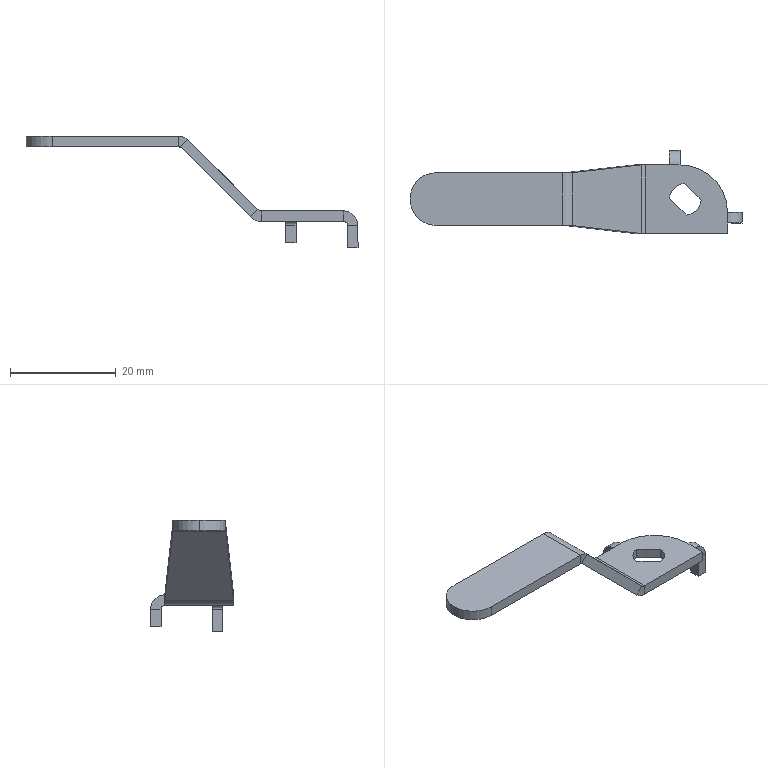Part | SolidWorks | features EdgeFlange 4, Fillet 2, ICE 2, FlatPattern 1, SMBaseFlange 1, SheetMetal 1 | 1 solid | 48 faces | box 62.879 x 15.737 x 21.142 mm | volume 1428 mm3 | plane 35 | cylinder 13 | commonest cylinder face diameters 1.473 x3 5.473 x3 6 x3 10 x2 2 x1 18 x1
STEP:
#1=CARTESIAN_POINT('',(-21.568,5.,13.544));
#2=VERTEX_POINT('',#1);
#3=CARTESIAN_POINT('',(-21.556,5.,13.556));
#4=VERTEX_POINT('',#3);
#5=CARTESIAN_POINT('',(-32.543,5.,2.57));
#6=DIRECTION('',(0.7071,0.,0.7071));
#7=VECTOR('',#6,1000.);
#8=LINE('',#5,#7);
#9=EDGE_CURVE('',#2,#4,#8,.T.);
#10=ORIENTED_EDGE('',*,*,#9,.F.);
#11=CARTESIAN_POINT('',(-21.341,5.,13.341));
#12=VERTEX_POINT('',#11);
#13=CARTESIAN_POINT('',(-23.276,5.,11.406));
#14=DIRECTION('',(0.,1.,0.));
#15=DIRECTION('',(0.,0.,1.));
#16=AXIS2_PLACEMENT_3D('',#13,#14,#15);
#17=CIRCLE('',#16,2.737);
#18=EDGE_CURVE('',#2,#12,#17,.T.);
#19=ORIENTED_EDGE('',*,*,#18,.T.);
#20=CARTESIAN_POINT('',(-4.,5.,-4.));
#21=DIRECTION('',(-0.7071,0.,0.7071));
#22=VECTOR('',#21,1000.);
#23=LINE('',#20,#22);
#24=EDGE_CURVE('',#12,#4,#23,.T.);
#25=ORIENTED_EDGE('',*,*,#24,.T.);
#26=EDGE_LOOP('',(#10,#19,#25));
#27=FACE_OUTER_BOUND('',#26,.T.);
#28=CARTESIAN_POINT('',(-22.971,5.,12.142));
#29=DIRECTION('',(0.,-1.,0.));
#30=DIRECTION('',(0.,0.,-1.));
#31=AXIS2_PLACEMENT_3D('',#28,#29,#30);
#32=PLANE('',#31);
#33=ADVANCED_FACE('',(#27),#32,.T.);
#34=CARTESIAN_POINT('',(-21.556,-5.,13.556));
#35=VERTEX_POINT('',#34);
#36=CARTESIAN_POINT('',(-21.341,-5.,13.341));
#37=VERTEX_POINT('',#36);
#38=CARTESIAN_POINT('',(-4.,-5.,-4.));
#39=DIRECTION('',(0.7071,0.,-0.7071));
#40=VECTOR('',#39,1000.);
#41=LINE('',#38,#40);
#42=EDGE_CURVE('',#35,#37,#41,.T.);
#43=ORIENTED_EDGE('',*,*,#42,.T.);
#44=CARTESIAN_POINT('',(-21.568,-5.,13.544));
#45=VERTEX_POINT('',#44);
#46=CARTESIAN_POINT('',(-23.276,-5.,11.406));
#47=DIRECTION('',(0.,-1.,0.));
#48=DIRECTION('',(0.,0.,1.));
#49=AXIS2_PLACEMENT_3D('',#46,#47,#48);
#50=CIRCLE('',#49,2.737);
#51=EDGE_CURVE('',#37,#45,#50,.T.);
#52=ORIENTED_EDGE('',*,*,#51,.T.);
#53=CARTESIAN_POINT('',(-32.543,-5.,2.57));
#54=DIRECTION('',(0.7071,0.,0.7071));
#55=VECTOR('',#54,1000.);
#56=LINE('',#53,#55);
#57=EDGE_CURVE('',#45,#35,#56,.T.);
#58=ORIENTED_EDGE('',*,*,#57,.T.);
#59=EDGE_LOOP('',(#43,#52,#58));
#60=FACE_OUTER_BOUND('',#59,.T.);
#61=CARTESIAN_POINT('',(-22.755,-5.,11.926));
#62=DIRECTION('',(0.,1.,0.));
#63=DIRECTION('',(0.,0.,1.));
#64=AXIS2_PLACEMENT_3D('',#61,#62,#63);
#65=PLANE('',#64);
#66=ADVANCED_FACE('',(#60),#65,.T.);
#67=CARTESIAN_POINT('',(-22.755,5.,11.926));
#68=VERTEX_POINT('',#67);
#69=CARTESIAN_POINT('',(-22.755,-5.,11.926));
#70=VERTEX_POINT('',#69);
#71=CARTESIAN_POINT('',(-22.755,5.,11.926));
#72=DIRECTION('',(0.,-1.,0.));
#73=VECTOR('',#72,1000.);
#74=LINE('',#71,#73);
#75=EDGE_CURVE('',#68,#70,#74,.T.);
#76=ORIENTED_EDGE('',*,*,#75,.F.);
#77=CARTESIAN_POINT('',(-22.971,5.,12.142));
#78=VERTEX_POINT('',#77);
#79=CARTESIAN_POINT('',(-22.971,5.,12.142));
#80=DIRECTION('',(0.7071,0.,-0.7071));
#81=VECTOR('',#80,1000.);
#82=LINE('',#79,#81);
#83=EDGE_CURVE('',#78,#68,#82,.T.);
#84=ORIENTED_EDGE('',*,*,#83,.F.);
#85=CARTESIAN_POINT('',(-9.707,6.5,-1.121));
#86=VERTEX_POINT('',#85);
#87=CARTESIAN_POINT('',(-9.707,6.5,-1.121));
#88=DIRECTION('',(0.7049,0.07971,-0.7049));
#89=VECTOR('',#88,1000.);
#90=LINE('',#87,#89);
#91=EDGE_CURVE('',#78,#86,#90,.T.);
#92=ORIENTED_EDGE('',*,*,#91,.T.);
#93=CARTESIAN_POINT('',(-9.707,-6.5,-1.121));
#94=VERTEX_POINT('',#93);
#95=CARTESIAN_POINT('',(-9.707,0.,-1.121));
#96=DIRECTION('',(0.,-1.,0.));
#97=VECTOR('',#96,1000.);
#98=LINE('',#95,#97);
#99=EDGE_CURVE('',#86,#94,#98,.T.);
#100=ORIENTED_EDGE('',*,*,#99,.T.);
#101=CARTESIAN_POINT('',(-22.971,-5.,12.142));
#102=VERTEX_POINT('',#101);
#103=CARTESIAN_POINT('',(-9.707,-6.5,-1.121));
#104=DIRECTION('',(-0.7049,0.07971,0.7049));
#105=VECTOR('',#104,1000.);
#106=LINE('',#103,#105);
#107=EDGE_CURVE('',#94,#102,#106,.T.);
#108=ORIENTED_EDGE('',*,*,#107,.T.);
#109=CARTESIAN_POINT('',(-22.755,-5.,11.926));
#110=DIRECTION('',(-0.7071,0.,0.7071));
#111=VECTOR('',#110,1000.);
#112=LINE('',#109,#111);
#113=EDGE_CURVE('',#70,#102,#112,.T.);
#114=ORIENTED_EDGE('',*,*,#113,.F.);
#115=EDGE_LOOP('',(#76,#84,#92,#100,#108,#114));
#116=FACE_OUTER_BOUND('',#115,.T.);
#117=CARTESIAN_POINT('',(-5.414,0.,-5.414));
#118=DIRECTION('',(-0.7071,0.,-0.7071));
#119=DIRECTION('',(-0.7071,0.,0.7071));
#120=AXIS2_PLACEMENT_3D('',#117,#118,#119);
#121=PLANE('',#120);
#122=ADVANCED_FACE('',(#116),#121,.T.);
#123=ORIENTED_EDGE('',*,*,#24,.F.);
#124=CARTESIAN_POINT('',(-21.341,5.,13.341));
#125=DIRECTION('',(0.,-1.,0.));
#126=VECTOR('',#125,1000.);
#127=LINE('',#124,#126);
#128=EDGE_CURVE('',#12,#37,#127,.T.);
#129=ORIENTED_EDGE('',*,*,#128,.T.);
#130=ORIENTED_EDGE('',*,*,#42,.F.);
#131=CARTESIAN_POINT('',(-8.293,-6.5,0.2929));
#132=VERTEX_POINT('',#131);
#133=CARTESIAN_POINT('',(-8.293,-6.5,0.2929));
#134=DIRECTION('',(-0.7049,0.07971,0.7049));
#135=VECTOR('',#134,1000.);
#136=LINE('',#133,#135);
#137=EDGE_CURVE('',#132,#35,#136,.T.);
#138=ORIENTED_EDGE('',*,*,#137,.F.);
#139=CARTESIAN_POINT('',(-8.293,6.5,0.2929));
#140=VERTEX_POINT('',#139);
#141=CARTESIAN_POINT('',(-8.293,6.5,0.2929));
#142=DIRECTION('',(0.,-1.,0.));
#143=VECTOR('',#142,1000.);
#144=LINE('',#141,#143);
#145=EDGE_CURVE('',#140,#132,#144,.T.);
#146=ORIENTED_EDGE('',*,*,#145,.F.);
#147=CARTESIAN_POINT('',(-8.293,6.5,0.2929));
#148=DIRECTION('',(0.7049,0.07971,-0.7049));
#149=VECTOR('',#148,1000.);
#150=LINE('',#147,#149);
#151=EDGE_CURVE('',#4,#140,#150,.T.);
#152=ORIENTED_EDGE('',*,*,#151,.F.);
#153=EDGE_LOOP('',(#123,#129,#130,#138,#146,#152));
#154=FACE_OUTER_BOUND('',#153,.T.);
#155=CARTESIAN_POINT('',(-4.,0.,-4.));
#156=DIRECTION('',(-0.7071,0.,-0.7071));
#157=DIRECTION('',(-0.7071,0.,0.7071));
#158=AXIS2_PLACEMENT_3D('',#155,#156,#157);
#159=PLANE('',#158);
#160=ADVANCED_FACE('',(#154),#159,.F.);
#161=CARTESIAN_POINT('',(-7.586,-6.5,0.));
#162=VERTEX_POINT('',#161);
#163=CARTESIAN_POINT('',(8.,-6.5,0.));
#164=VERTEX_POINT('',#163);
#165=CARTESIAN_POINT('',(-8.,-6.5,0.));
#166=DIRECTION('',(1.,0.,0.));
#167=VECTOR('',#166,1000.);
#168=LINE('',#165,#167);
#169=EDGE_CURVE('',#162,#164,#168,.T.);
#170=ORIENTED_EDGE('',*,*,#169,.F.);
#171=CARTESIAN_POINT('',(-7.586,-6.5,-2.));
#172=VERTEX_POINT('',#171);
#173=CARTESIAN_POINT('',(-7.586,-6.5,0.));
#174=DIRECTION('',(0.,0.,-1.));
#175=VECTOR('',#174,1000.);
#176=LINE('',#173,#175);
#177=EDGE_CURVE('',#162,#172,#176,.T.);
#178=ORIENTED_EDGE('',*,*,#177,.T.);
#179=CARTESIAN_POINT('',(8.,-6.5,-2.));
#180=VERTEX_POINT('',#179);
#181=CARTESIAN_POINT('',(-8.,-6.5,-2.));
#182=DIRECTION('',(1.,0.,0.));
#183=VECTOR('',#182,1000.);
#184=LINE('',#181,#183);
#185=EDGE_CURVE('',#172,#180,#184,.T.);
#186=ORIENTED_EDGE('',*,*,#185,.T.);
#187=CARTESIAN_POINT('',(8.,-6.5,-2.));
#188=DIRECTION('',(0.,0.,1.));
#189=VECTOR('',#188,1000.);
#190=LINE('',#187,#189);
#191=EDGE_CURVE('',#180,#164,#190,.T.);
#192=ORIENTED_EDGE('',*,*,#191,.T.);
#193=EDGE_LOOP('',(#170,#178,#186,#192));
#194=FACE_OUTER_BOUND('',#193,.T.);
#195=CARTESIAN_POINT('',(-8.,-6.5,-2.));
#196=DIRECTION('',(0.,-1.,0.));
#197=DIRECTION('',(0.,0.,-1.));
#198=AXIS2_PLACEMENT_3D('',#195,#196,#197);
#199=PLANE('',#198);
#200=ADVANCED_FACE('',(#194),#199,.T.);
#201=CARTESIAN_POINT('',(-0.1669,2.995,-2.));
#202=VERTEX_POINT('',#201);
#203=CARTESIAN_POINT('',(2.995,-0.1669,-2.));
#204=VERTEX_POINT('',#203);
#205=CARTESIAN_POINT('',(-0.1669,2.995,-2.));
#206=DIRECTION('',(0.7071,-0.7071,0.));
#207=VECTOR('',#206,1000.);
#208=LINE('',#205,#207);
#209=EDGE_CURVE('',#202,#204,#208,.T.);
#210=ORIENTED_EDGE('',*,*,#209,.F.);
#211=CARTESIAN_POINT('',(-2.995,0.1669,-2.));
#212=VERTEX_POINT('',#211);
#213=CARTESIAN_POINT('',(0.,0.,-2.));
#214=DIRECTION('',(0.,0.,-1.));
#215=DIRECTION('',(1.,0.,0.));
#216=AXIS2_PLACEMENT_3D('',#213,#214,#215);
#217=CIRCLE('',#216,3.);
#218=EDGE_CURVE('',#212,#202,#217,.T.);
#219=ORIENTED_EDGE('',*,*,#218,.F.);
#220=CARTESIAN_POINT('',(0.1669,-2.995,-2.));
#221=VERTEX_POINT('',#220);
#222=CARTESIAN_POINT('',(-2.995,0.1669,-2.));
#223=DIRECTION('',(-0.7071,0.7071,0.));
#224=VECTOR('',#223,1000.);
#225=LINE('',#222,#224);
#226=EDGE_CURVE('',#221,#212,#225,.T.);
#227=ORIENTED_EDGE('',*,*,#226,.F.);
#228=CARTESIAN_POINT('',(0.,0.,-2.));
#229=DIRECTION('',(0.,0.,-1.));
#230=DIRECTION('',(1.,0.,0.));
#231=AXIS2_PLACEMENT_3D('',#228,#229,#230);
#232=CIRCLE('',#231,3.);
#233=EDGE_CURVE('',#204,#221,#232,.T.);
#234=ORIENTED_EDGE('',*,*,#233,.F.);
#235=EDGE_LOOP('',(#210,#219,#227,#234));
#236=FACE_BOUND('',#235,.T.);
#237=CARTESIAN_POINT('',(-1.,6.5,-2.));
#238=VERTEX_POINT('',#237);
#239=CARTESIAN_POINT('',(-3.,6.5,-2.));
#240=VERTEX_POINT('',#239);
#241=CARTESIAN_POINT('',(-1.,6.5,-2.));
#242=DIRECTION('',(-1.,0.,0.));
#243=VECTOR('',#242,1000.);
#244=LINE('',#241,#243);
#245=EDGE_CURVE('',#238,#240,#244,.T.);
#246=ORIENTED_EDGE('',*,*,#245,.F.);
#247=CARTESIAN_POINT('',(8.,-2.5,-2.));
#248=VERTEX_POINT('',#247);
#249=CARTESIAN_POINT('',(-1.,-2.5,-2.));
#250=DIRECTION('',(0.,0.,-1.));
#251=DIRECTION('',(1.,0.,0.));
#252=AXIS2_PLACEMENT_3D('',#249,#250,#251);
#253=CIRCLE('',#252,9.);
#254=EDGE_CURVE('',#238,#248,#253,.T.);
#255=ORIENTED_EDGE('',*,*,#254,.T.);
#256=CARTESIAN_POINT('',(8.,-4.5,-2.));
#257=VERTEX_POINT('',#256);
#258=CARTESIAN_POINT('',(8.,-4.5,-2.));
#259=DIRECTION('',(0.,1.,0.));
#260=VECTOR('',#259,1000.);
#261=LINE('',#258,#260);
#262=EDGE_CURVE('',#257,#248,#261,.T.);
#263=ORIENTED_EDGE('',*,*,#262,.F.);
#264=CARTESIAN_POINT('',(8.,6.5,-2.));
#265=DIRECTION('',(0.,1.,0.));
#266=VECTOR('',#265,1000.);
#267=LINE('',#264,#266);
#268=EDGE_CURVE('',#180,#257,#267,.T.);
#269=ORIENTED_EDGE('',*,*,#268,.F.);
#270=ORIENTED_EDGE('',*,*,#185,.F.);
#271=CARTESIAN_POINT('',(-7.586,6.5,-2.));
#272=VERTEX_POINT('',#271);
#273=CARTESIAN_POINT('',(-7.586,-6.5,-2.));
#274=DIRECTION('',(0.,1.,0.));
#275=VECTOR('',#274,1000.);
#276=LINE('',#273,#275);
#277=EDGE_CURVE('',#172,#272,#276,.T.);
#278=ORIENTED_EDGE('',*,*,#277,.T.);
#279=CARTESIAN_POINT('',(-8.,6.5,-2.));
#280=DIRECTION('',(-1.,0.,0.));
#281=VECTOR('',#280,1000.);
#282=LINE('',#279,#281);
#283=EDGE_CURVE('',#240,#272,#282,.T.);
#284=ORIENTED_EDGE('',*,*,#283,.F.);
#285=EDGE_LOOP('',(#246,#255,#263,#269,#270,#278,#284));
#286=FACE_OUTER_BOUND('',#285,.T.);
#287=CARTESIAN_POINT('',(0.,0.,-2.));
#288=DIRECTION('',(0.,0.,1.));
#289=DIRECTION('',(1.,0.,0.));
#290=AXIS2_PLACEMENT_3D('',#287,#288,#289);
#291=PLANE('',#290);
#292=ADVANCED_FACE('',(#236,#286),#291,.F.);
#293=CARTESIAN_POINT('',(-0.1669,2.995,0.));
#294=VERTEX_POINT('',#293);
#295=CARTESIAN_POINT('',(-2.995,0.1669,0.));
#296=VERTEX_POINT('',#295);
#297=CARTESIAN_POINT('',(0.,0.,0.));
#298=DIRECTION('',(0.,0.,1.));
#299=DIRECTION('',(1.,0.,0.));
#300=AXIS2_PLACEMENT_3D('',#297,#298,#299);
#301=CIRCLE('',#300,3.);
#302=EDGE_CURVE('',#294,#296,#301,.T.);
#303=ORIENTED_EDGE('',*,*,#302,.F.);
#304=CARTESIAN_POINT('',(2.995,-0.1669,0.));
#305=VERTEX_POINT('',#304);
#306=CARTESIAN_POINT('',(-0.1669,2.995,0.));
#307=DIRECTION('',(-0.7071,0.7071,0.));
#308=VECTOR('',#307,1000.);
#309=LINE('',#306,#308);
#310=EDGE_CURVE('',#305,#294,#309,.T.);
#311=ORIENTED_EDGE('',*,*,#310,.F.);
#312=CARTESIAN_POINT('',(0.1669,-2.995,0.));
#313=VERTEX_POINT('',#312);
#314=CARTESIAN_POINT('',(0.,0.,0.));
#315=DIRECTION('',(0.,0.,1.));
#316=DIRECTION('',(1.,0.,0.));
#317=AXIS2_PLACEMENT_3D('',#314,#315,#316);
#318=CIRCLE('',#317,3.);
#319=EDGE_CURVE('',#313,#305,#318,.T.);
#320=ORIENTED_EDGE('',*,*,#319,.F.);
#321=CARTESIAN_POINT('',(-2.995,0.1669,0.));
#322=DIRECTION('',(0.7071,-0.7071,0.));
#323=VECTOR('',#322,1000.);
#324=LINE('',#321,#323);
#325=EDGE_CURVE('',#296,#313,#324,.T.);
#326=ORIENTED_EDGE('',*,*,#325,.F.);
#327=EDGE_LOOP('',(#303,#311,#320,#326));
#328=FACE_BOUND('',#327,.T.);
#329=CARTESIAN_POINT('',(8.,-4.5,0.));
#330=VERTEX_POINT('',#329);
#331=CARTESIAN_POINT('',(8.,-2.5,0.));
#332=VERTEX_POINT('',#331);
#333=CARTESIAN_POINT('',(8.,-4.5,0.));
#334=DIRECTION('',(0.,1.,0.));
#335=VECTOR('',#334,1000.);
#336=LINE('',#333,#335);
#337=EDGE_CURVE('',#330,#332,#336,.T.);
#338=ORIENTED_EDGE('',*,*,#337,.T.);
#339=CARTESIAN_POINT('',(-1.,6.5,0.));
#340=VERTEX_POINT('',#339);
#341=CARTESIAN_POINT('',(-1.,-2.5,0.));
#342=DIRECTION('',(0.,0.,1.));
#343=DIRECTION('',(1.,0.,0.));
#344=AXIS2_PLACEMENT_3D('',#341,#342,#343);
#345=CIRCLE('',#344,9.);
#346=EDGE_CURVE('',#332,#340,#345,.T.);
#347=ORIENTED_EDGE('',*,*,#346,.T.);
#348=CARTESIAN_POINT('',(-3.,6.5,0.));
#349=VERTEX_POINT('',#348);
#350=CARTESIAN_POINT('',(-1.,6.5,0.));
#351=DIRECTION('',(-1.,0.,0.));
#352=VECTOR('',#351,1000.);
#353=LINE('',#350,#352);
#354=EDGE_CURVE('',#340,#349,#353,.T.);
#355=ORIENTED_EDGE('',*,*,#354,.T.);
#356=CARTESIAN_POINT('',(-7.586,6.5,0.));
#357=VERTEX_POINT('',#356);
#358=CARTESIAN_POINT('',(-8.,6.5,0.));
#359=DIRECTION('',(-1.,0.,0.));
#360=VECTOR('',#359,1000.);
#361=LINE('',#358,#360);
#362=EDGE_CURVE('',#349,#357,#361,.T.);
#363=ORIENTED_EDGE('',*,*,#362,.T.);
#364=CARTESIAN_POINT('',(-7.586,-6.5,0.));
#365=DIRECTION('',(0.,1.,0.));
#366=VECTOR('',#365,1000.);
#367=LINE('',#364,#366);
#368=EDGE_CURVE('',#162,#357,#367,.T.);
#369=ORIENTED_EDGE('',*,*,#368,.F.);
#370=ORIENTED_EDGE('',*,*,#169,.T.);
#371=CARTESIAN_POINT('',(8.,6.5,0.));
#372=DIRECTION('',(0.,1.,0.));
#373=VECTOR('',#372,1000.);
#374=LINE('',#371,#373);
#375=EDGE_CURVE('',#164,#330,#374,.T.);
#376=ORIENTED_EDGE('',*,*,#375,.T.);
#377=EDGE_LOOP('',(#338,#347,#355,#363,#369,#370,#376));
#378=FACE_OUTER_BOUND('',#377,.T.);
#379=CARTESIAN_POINT('',(0.,0.,0.));
#380=DIRECTION('',(0.,0.,1.));
#381=DIRECTION('',(1.,0.,0.));
#382=AXIS2_PLACEMENT_3D('',#379,#380,#381);
#383=PLANE('',#382);
#384=ADVANCED_FACE('',(#328,#378),#383,.T.);
#385=ORIENTED_EDGE('',*,*,#268,.T.);
#386=CARTESIAN_POINT('',(8.,-4.5,-2.));
#387=DIRECTION('',(0.,0.,1.));
#388=VECTOR('',#387,1000.);
#389=LINE('',#386,#388);
#390=EDGE_CURVE('',#257,#330,#389,.T.);
#391=ORIENTED_EDGE('',*,*,#390,.T.);
#392=ORIENTED_EDGE('',*,*,#375,.F.);
#393=ORIENTED_EDGE('',*,*,#191,.F.);
#394=EDGE_LOOP('',(#385,#391,#392,#393));
#395=FACE_OUTER_BOUND('',#394,.T.);
#396=CARTESIAN_POINT('',(8.,6.5,-2.));
#397=DIRECTION('',(1.,0.,0.));
#398=DIRECTION('',(0.,1.,0.));
#399=AXIS2_PLACEMENT_3D('',#396,#397,#398);
#400=PLANE('',#399);
#401=ADVANCED_FACE('',(#395),#400,.T.);
#402=CARTESIAN_POINT('',(-7.586,6.5,0.));
#403=DIRECTION('',(0.,0.,-1.));
#404=VECTOR('',#403,1000.);
#405=LINE('',#402,#404);
#406=EDGE_CURVE('',#357,#272,#405,.T.);
#407=ORIENTED_EDGE('',*,*,#406,.F.);
#408=ORIENTED_EDGE('',*,*,#362,.F.);
#409=CARTESIAN_POINT('',(-3.,6.5,-2.));
#410=DIRECTION('',(0.,0.,1.));
#411=VECTOR('',#410,1000.);
#412=LINE('',#409,#411);
#413=EDGE_CURVE('',#240,#349,#412,.T.);
#414=ORIENTED_EDGE('',*,*,#413,.F.);
#415=ORIENTED_EDGE('',*,*,#283,.T.);
#416=EDGE_LOOP('',(#407,#408,#414,#415));
#417=FACE_OUTER_BOUND('',#416,.T.);
#418=CARTESIAN_POINT('',(-8.,6.5,-2.));
#419=DIRECTION('',(0.,1.,0.));
#420=DIRECTION('',(-1.,0.,0.));
#421=AXIS2_PLACEMENT_3D('',#418,#419,#420);
#422=PLANE('',#421);
#423=ADVANCED_FACE('',(#417),#422,.T.);
#424=CARTESIAN_POINT('',(8.737,-2.5,-2.737));
#425=VERTEX_POINT('',#424);
#426=CARTESIAN_POINT('',(10.737,-2.5,-2.737));
#427=VERTEX_POINT('',#426);
#428=CARTESIAN_POINT('',(10.737,-2.5,-2.737));
#429=DIRECTION('',(1.,0.,0.));
#430=VECTOR('',#429,1000.);
#431=LINE('',#428,#430);
#432=EDGE_CURVE('',#425,#427,#431,.T.);
#433=ORIENTED_EDGE('',*,*,#432,.F.);
#434=CARTESIAN_POINT('',(8.,-2.5,-2.737));
#435=DIRECTION('',(0.,1.,0.));
#436=DIRECTION('',(0.,0.,-1.));
#437=AXIS2_PLACEMENT_3D('',#434,#435,#436);
#438=CIRCLE('',#437,0.7366);
#439=EDGE_CURVE('',#248,#425,#438,.T.);
#440=ORIENTED_EDGE('',*,*,#439,.F.);
#441=CARTESIAN_POINT('',(8.,-2.5,-2.));
#442=DIRECTION('',(0.,0.,1.));
#443=VECTOR('',#442,1000.);
#444=LINE('',#441,#443);
#445=EDGE_CURVE('',#248,#332,#444,.T.);
#446=ORIENTED_EDGE('',*,*,#445,.T.);
#447=CARTESIAN_POINT('',(8.,-2.5,-2.737));
#448=DIRECTION('',(0.,1.,0.));
#449=DIRECTION('',(0.,0.,-1.));
#450=AXIS2_PLACEMENT_3D('',#447,#448,#449);
#451=CIRCLE('',#450,2.737);
#452=EDGE_CURVE('',#332,#427,#451,.T.);
#453=ORIENTED_EDGE('',*,*,#452,.T.);
#454=EDGE_LOOP('',(#433,#440,#446,#453));
#455=FACE_OUTER_BOUND('',#454,.T.);
#456=CARTESIAN_POINT('',(8.,-2.5,-2.737));
#457=DIRECTION('',(0.,1.,0.));
#458=DIRECTION('',(0.,0.,1.));
#459=AXIS2_PLACEMENT_3D('',#456,#457,#458);
#460=PLANE('',#459);
#461=ADVANCED_FACE('',(#455),#460,.T.);
#462=CARTESIAN_POINT('',(8.737,-4.5,-2.737));
#463=VERTEX_POINT('',#462);
#464=CARTESIAN_POINT('',(8.,-4.5,-2.737));
#465=DIRECTION('',(0.,-1.,0.));
#466=DIRECTION('',(0.,0.,-1.));
#467=AXIS2_PLACEMENT_3D('',#464,#465,#466);
#468=CIRCLE('',#467,0.7366);
#469=EDGE_CURVE('',#463,#257,#468,.T.);
#470=ORIENTED_EDGE('',*,*,#469,.F.);
#471=CARTESIAN_POINT('',(10.737,-4.5,-2.737));
#472=VERTEX_POINT('',#471);
#473=CARTESIAN_POINT('',(8.737,-4.5,-2.737));
#474=DIRECTION('',(1.,0.,0.));
#475=VECTOR('',#474,1000.);
#476=LINE('',#473,#475);
#477=EDGE_CURVE('',#463,#472,#476,.T.);
#478=ORIENTED_EDGE('',*,*,#477,.T.);
#479=CARTESIAN_POINT('',(8.,-4.5,-2.737));
#480=DIRECTION('',(0.,-1.,0.));
#481=DIRECTION('',(0.,0.,-1.));
#482=AXIS2_PLACEMENT_3D('',#479,#480,#481);
#483=CIRCLE('',#482,2.737);
#484=EDGE_CURVE('',#472,#330,#483,.T.);
#485=ORIENTED_EDGE('',*,*,#484,.T.);
#486=ORIENTED_EDGE('',*,*,#390,.F.);
#487=EDGE_LOOP('',(#470,#478,#485,#486));
#488=FACE_OUTER_BOUND('',#487,.T.);
#489=CARTESIAN_POINT('',(8.,-4.5,-2.737));
#490=DIRECTION('',(0.,1.,0.));
#491=DIRECTION('',(0.,0.,1.));
#492=AXIS2_PLACEMENT_3D('',#489,#490,#491);
#493=PLANE('',#492);
#494=ADVANCED_FACE('',(#488),#493,.F.);
#495=ORIENTED_EDGE('',*,*,#337,.F.);
#496=ORIENTED_EDGE('',*,*,#484,.F.);
#497=CARTESIAN_POINT('',(10.737,0.,-2.737));
#498=DIRECTION('',(0.,-1.,0.));
#499=VECTOR('',#498,1000.);
#500=LINE('',#497,#499);
#501=EDGE_CURVE('',#427,#472,#500,.T.);
#502=ORIENTED_EDGE('',*,*,#501,.F.);
#503=ORIENTED_EDGE('',*,*,#452,.F.);
#504=EDGE_LOOP('',(#495,#496,#502,#503));
#505=FACE_OUTER_BOUND('',#504,.T.);
#506=CARTESIAN_POINT('',(8.,-4.5,-2.737));
#507=DIRECTION('',(0.,-1.,0.));
#508=DIRECTION('',(1.,0.,0.));
#509=AXIS2_PLACEMENT_3D('',#506,#507,#508);
#510=CYLINDRICAL_SURFACE('',#509,2.737);
#511=ADVANCED_FACE('',(#505),#510,.T.);
#512=ORIENTED_EDGE('',*,*,#262,.T.);
#513=ORIENTED_EDGE('',*,*,#439,.T.);
#514=CARTESIAN_POINT('',(8.737,-2.5,-2.737));
#515=DIRECTION('',(0.,-1.,0.));
#516=VECTOR('',#515,1000.);
#517=LINE('',#514,#516);
#518=EDGE_CURVE('',#425,#463,#517,.T.);
#519=ORIENTED_EDGE('',*,*,#518,.T.);
#520=ORIENTED_EDGE('',*,*,#469,.T.);
#521=EDGE_LOOP('',(#512,#513,#519,#520));
#522=FACE_OUTER_BOUND('',#521,.T.);
#523=CARTESIAN_POINT('',(8.,-4.5,-2.737));
#524=DIRECTION('',(0.,-1.,0.));
#525=DIRECTION('',(1.,0.,0.));
#526=AXIS2_PLACEMENT_3D('',#523,#524,#525);
#527=CYLINDRICAL_SURFACE('',#526,0.7366);
#528=ADVANCED_FACE('',(#522),#527,.F.);
#529=CARTESIAN_POINT('',(10.737,-4.5,-7.));
#530=VERTEX_POINT('',#529);
#531=CARTESIAN_POINT('',(10.737,-4.5,-2.));
#532=DIRECTION('',(0.,0.,1.));
#533=VECTOR('',#532,1000.);
#534=LINE('',#531,#533);
#535=EDGE_CURVE('',#530,#472,#534,.T.);
#536=ORIENTED_EDGE('',*,*,#535,.T.);
#537=ORIENTED_EDGE('',*,*,#477,.F.);
#538=CARTESIAN_POINT('',(8.737,-4.5,-7.));
#539=VERTEX_POINT('',#538);
#540=CARTESIAN_POINT('',(8.737,-4.5,0.));
#541=DIRECTION('',(0.,0.,1.));
#542=VECTOR('',#541,1000.);
#543=LINE('',#540,#542);
#544=EDGE_CURVE('',#539,#463,#543,.T.);
#545=ORIENTED_EDGE('',*,*,#544,.F.);
#546=CARTESIAN_POINT('',(10.737,-4.5,-7.));
#547=DIRECTION('',(-1.,0.,0.));
#548=VECTOR('',#547,1000.);
#549=LINE('',#546,#548);
#550=EDGE_CURVE('',#530,#539,#549,.T.);
#551=ORIENTED_EDGE('',*,*,#550,.F.);
#552=EDGE_LOOP('',(#536,#537,#545,#551));
#553=FACE_OUTER_BOUND('',#552,.T.);
#554=CARTESIAN_POINT('',(10.737,-4.5,-2.));
#555=DIRECTION('',(0.,-1.,0.));
#556=DIRECTION('',(1.,0.,0.));
#557=AXIS2_PLACEMENT_3D('',#554,#555,#556);
#558=PLANE('',#557);
#559=ADVANCED_FACE('',(#553),#558,.T.);
#560=CARTESIAN_POINT('',(8.737,-2.5,-7.));
#561=VERTEX_POINT('',#560);
#562=CARTESIAN_POINT('',(8.737,-2.5,0.));
#563=DIRECTION('',(0.,0.,-1.));
#564=VECTOR('',#563,1000.);
#565=LINE('',#562,#564);
#566=EDGE_CURVE('',#425,#561,#565,.T.);
#567=ORIENTED_EDGE('',*,*,#566,.F.);
#568=ORIENTED_EDGE('',*,*,#432,.T.);
#569=CARTESIAN_POINT('',(10.737,-2.5,-7.));
#570=VERTEX_POINT('',#569);
#571=CARTESIAN_POINT('',(10.737,-2.5,-7.));
#572=DIRECTION('',(0.,0.,-1.));
#573=VECTOR('',#572,1000.);
#574=LINE('',#571,#573);
#575=EDGE_CURVE('',#427,#570,#574,.T.);
#576=ORIENTED_EDGE('',*,*,#575,.T.);
#577=CARTESIAN_POINT('',(10.737,-2.5,-7.));
#578=DIRECTION('',(-1.,0.,0.));
#579=VECTOR('',#578,1000.);
#580=LINE('',#577,#579);
#581=EDGE_CURVE('',#570,#561,#580,.T.);
#582=ORIENTED_EDGE('',*,*,#581,.T.);
#583=EDGE_LOOP('',(#567,#568,#576,#582));
#584=FACE_OUTER_BOUND('',#583,.T.);
#585=CARTESIAN_POINT('',(10.737,-2.5,-7.));
#586=DIRECTION('',(0.,1.,0.));
#587=DIRECTION('',(-1.,0.,0.));
#588=AXIS2_PLACEMENT_3D('',#585,#586,#587);
#589=PLANE('',#588);
#590=ADVANCED_FACE('',(#584),#589,.T.);
#591=ORIENTED_EDGE('',*,*,#575,.F.);
#592=ORIENTED_EDGE('',*,*,#501,.T.);
#593=ORIENTED_EDGE('',*,*,#535,.F.);
#594=CARTESIAN_POINT('',(10.737,-4.5,-7.));
#595=DIRECTION('',(0.,-1.,0.));
#596=VECTOR('',#595,1000.);
#597=LINE('',#594,#596);
#598=EDGE_CURVE('',#570,#530,#597,.T.);
#599=ORIENTED_EDGE('',*,*,#598,.F.);
#600=EDGE_LOOP('',(#591,#592,#593,#599));
#601=FACE_OUTER_BOUND('',#600,.T.);
#602=CARTESIAN_POINT('',(10.737,0.,0.));
#603=DIRECTION('',(1.,0.,0.));
#604=DIRECTION('',(0.,0.,-1.));
#605=AXIS2_PLACEMENT_3D('',#602,#603,#604);
#606=PLANE('',#605);
#607=ADVANCED_FACE('',(#601),#606,.T.);
#608=ORIENTED_EDGE('',*,*,#518,.F.);
#609=ORIENTED_EDGE('',*,*,#566,.T.);
#610=CARTESIAN_POINT('',(8.737,0.,-7.));
#611=DIRECTION('',(0.,-1.,0.));
#612=VECTOR('',#611,1000.);
#613=LINE('',#610,#612);
#614=EDGE_CURVE('',#561,#539,#613,.T.);
#615=ORIENTED_EDGE('',*,*,#614,.T.);
#616=ORIENTED_EDGE('',*,*,#544,.T.);
#617=EDGE_LOOP('',(#608,#609,#615,#616));
#618=FACE_OUTER_BOUND('',#617,.T.);
#619=CARTESIAN_POINT('',(8.737,0.,0.));
#620=DIRECTION('',(1.,0.,0.));
#621=DIRECTION('',(0.,0.,-1.));
#622=AXIS2_PLACEMENT_3D('',#619,#620,#621);
#623=PLANE('',#622);
#624=ADVANCED_FACE('',(#618),#623,.F.);
#625=ORIENTED_EDGE('',*,*,#614,.F.);
#626=ORIENTED_EDGE('',*,*,#581,.F.);
#627=ORIENTED_EDGE('',*,*,#598,.T.);
#628=ORIENTED_EDGE('',*,*,#550,.T.);
#629=EDGE_LOOP('',(#625,#626,#627,#628));
#630=FACE_OUTER_BOUND('',#629,.T.);
#631=CARTESIAN_POINT('',(10.737,-4.5,-7.));
#632=DIRECTION('',(0.,0.,-1.));
#633=DIRECTION('',(-1.,0.,0.));
#634=AXIS2_PLACEMENT_3D('',#631,#632,#633);
#635=PLANE('',#634);
#636=ADVANCED_FACE('',(#630),#635,.T.);
#637=CARTESIAN_POINT('',(-3.,7.237,-2.737));
#638=VERTEX_POINT('',#637);
#639=CARTESIAN_POINT('',(-3.,9.237,-2.737));
#640=VERTEX_POINT('',#639);
#641=CARTESIAN_POINT('',(-3.,9.237,-2.737));
#642=DIRECTION('',(0.,1.,0.));
#643=VECTOR('',#642,1000.);
#644=LINE('',#641,#643);
#645=EDGE_CURVE('',#638,#640,#644,.T.);
#646=ORIENTED_EDGE('',*,*,#645,.F.);
#647=CARTESIAN_POINT('',(-3.,6.5,-2.737));
#648=DIRECTION('',(-1.,0.,0.));
#649=DIRECTION('',(0.,0.,-1.));
#650=AXIS2_PLACEMENT_3D('',#647,#648,#649);
#651=CIRCLE('',#650,0.7366);
#652=EDGE_CURVE('',#240,#638,#651,.T.);
#653=ORIENTED_EDGE('',*,*,#652,.F.);
#654=ORIENTED_EDGE('',*,*,#413,.T.);
#655=CARTESIAN_POINT('',(-3.,6.5,-2.737));
#656=DIRECTION('',(-1.,0.,0.));
#657=DIRECTION('',(0.,0.,-1.));
#658=AXIS2_PLACEMENT_3D('',#655,#656,#657);
#659=CIRCLE('',#658,2.737);
#660=EDGE_CURVE('',#349,#640,#659,.T.);
#661=ORIENTED_EDGE('',*,*,#660,.T.);
#662=EDGE_LOOP('',(#646,#653,#654,#661));
#663=FACE_OUTER_BOUND('',#662,.T.);
#664=CARTESIAN_POINT('',(-3.,6.5,-2.737));
#665=DIRECTION('',(-1.,0.,0.));
#666=DIRECTION('',(0.,0.,1.));
#667=AXIS2_PLACEMENT_3D('',#664,#665,#666);
#668=PLANE('',#667);
#669=ADVANCED_FACE('',(#663),#668,.T.);
#670=CARTESIAN_POINT('',(-1.,7.237,-2.737));
#671=VERTEX_POINT('',#670);
#672=CARTESIAN_POINT('',(-1.,6.5,-2.737));
#673=DIRECTION('',(1.,0.,0.));
#674=DIRECTION('',(0.,0.,-1.));
#675=AXIS2_PLACEMENT_3D('',#672,#673,#674);
#676=CIRCLE('',#675,0.7366);
#677=EDGE_CURVE('',#671,#238,#676,.T.);
#678=ORIENTED_EDGE('',*,*,#677,.F.);
#679=CARTESIAN_POINT('',(-1.,9.237,-2.737));
#680=VERTEX_POINT('',#679);
#681=CARTESIAN_POINT('',(-1.,7.237,-2.737));
#682=DIRECTION('',(0.,1.,0.));
#683=VECTOR('',#682,1000.);
#684=LINE('',#681,#683);
#685=EDGE_CURVE('',#671,#680,#684,.T.);
#686=ORIENTED_EDGE('',*,*,#685,.T.);
#687=CARTESIAN_POINT('',(-1.,6.5,-2.737));
#688=DIRECTION('',(1.,0.,0.));
#689=DIRECTION('',(0.,0.,-1.));
#690=AXIS2_PLACEMENT_3D('',#687,#688,#689);
#691=CIRCLE('',#690,2.737);
#692=EDGE_CURVE('',#680,#340,#691,.T.);
#693=ORIENTED_EDGE('',*,*,#692,.T.);
#694=CARTESIAN_POINT('',(-1.,6.5,-2.));
#695=DIRECTION('',(0.,0.,1.));
#696=VECTOR('',#695,1000.);
#697=LINE('',#694,#696);
#698=EDGE_CURVE('',#238,#340,#697,.T.);
#699=ORIENTED_EDGE('',*,*,#698,.F.);
#700=EDGE_LOOP('',(#678,#686,#693,#699));
#701=FACE_OUTER_BOUND('',#700,.T.);
#702=CARTESIAN_POINT('',(-1.,6.5,-2.737));
#703=DIRECTION('',(-1.,0.,0.));
#704=DIRECTION('',(0.,0.,1.));
#705=AXIS2_PLACEMENT_3D('',#702,#703,#704);
#706=PLANE('',#705);
#707=ADVANCED_FACE('',(#701),#706,.F.);
#708=ORIENTED_EDGE('',*,*,#354,.F.);
#709=ORIENTED_EDGE('',*,*,#692,.F.);
#710=CARTESIAN_POINT('',(0.,9.237,-2.737));
#711=DIRECTION('',(1.,0.,0.));
#712=VECTOR('',#711,1000.);
#713=LINE('',#710,#712);
#714=EDGE_CURVE('',#640,#680,#713,.T.);
#715=ORIENTED_EDGE('',*,*,#714,.F.);
#716=ORIENTED_EDGE('',*,*,#660,.F.);
#717=EDGE_LOOP('',(#708,#709,#715,#716));
#718=FACE_OUTER_BOUND('',#717,.T.);
#719=CARTESIAN_POINT('',(-1.,6.5,-2.737));
#720=DIRECTION('',(1.,0.,0.));
#721=DIRECTION('',(0.,1.,0.));
#722=AXIS2_PLACEMENT_3D('',#719,#720,#721);
#723=CYLINDRICAL_SURFACE('',#722,2.737);
#724=ADVANCED_FACE('',(#718),#723,.T.);
#725=ORIENTED_EDGE('',*,*,#245,.T.);
#726=ORIENTED_EDGE('',*,*,#652,.T.);
#727=CARTESIAN_POINT('',(-3.,7.237,-2.737));
#728=DIRECTION('',(1.,0.,0.));
#729=VECTOR('',#728,1000.);
#730=LINE('',#727,#729);
#731=EDGE_CURVE('',#638,#671,#730,.T.);
#732=ORIENTED_EDGE('',*,*,#731,.T.);
#733=ORIENTED_EDGE('',*,*,#677,.T.);
#734=EDGE_LOOP('',(#725,#726,#732,#733));
#735=FACE_OUTER_BOUND('',#734,.T.);
#736=CARTESIAN_POINT('',(-1.,6.5,-2.737));
#737=DIRECTION('',(1.,0.,0.));
#738=DIRECTION('',(0.,1.,0.));
#739=AXIS2_PLACEMENT_3D('',#736,#737,#738);
#740=CYLINDRICAL_SURFACE('',#739,0.7366);
#741=ADVANCED_FACE('',(#735),#740,.F.);
#742=CARTESIAN_POINT('',(-1.,9.237,-6.));
#743=VERTEX_POINT('',#742);
#744=CARTESIAN_POINT('',(-1.,9.237,-2.));
#745=DIRECTION('',(0.,0.,1.));
#746=VECTOR('',#745,1000.);
#747=LINE('',#744,#746);
#748=EDGE_CURVE('',#743,#680,#747,.T.);
#749=ORIENTED_EDGE('',*,*,#748,.T.);
#750=ORIENTED_EDGE('',*,*,#685,.F.);
#751=CARTESIAN_POINT('',(-1.,7.237,-6.));
#752=VERTEX_POINT('',#751);
#753=CARTESIAN_POINT('',(-1.,7.237,0.));
#754=DIRECTION('',(0.,0.,1.));
#755=VECTOR('',#754,1000.);
#756=LINE('',#753,#755);
#757=EDGE_CURVE('',#752,#671,#756,.T.);
#758=ORIENTED_EDGE('',*,*,#757,.F.);
#759=CARTESIAN_POINT('',(-1.,9.237,-6.));
#760=DIRECTION('',(0.,-1.,0.));
#761=VECTOR('',#760,1000.);
#762=LINE('',#759,#761);
#763=EDGE_CURVE('',#743,#752,#762,.T.);
#764=ORIENTED_EDGE('',*,*,#763,.F.);
#765=EDGE_LOOP('',(#749,#750,#758,#764));
#766=FACE_OUTER_BOUND('',#765,.T.);
#767=CARTESIAN_POINT('',(-1.,9.237,-2.));
#768=DIRECTION('',(1.,0.,0.));
#769=DIRECTION('',(0.,1.,0.));
#770=AXIS2_PLACEMENT_3D('',#767,#768,#769);
#771=PLANE('',#770);
#772=ADVANCED_FACE('',(#766),#771,.T.);
#773=CARTESIAN_POINT('',(-3.,7.237,-6.));
#774=VERTEX_POINT('',#773);
#775=CARTESIAN_POINT('',(-3.,7.237,0.));
#776=DIRECTION('',(0.,0.,-1.));
#777=VECTOR('',#776,1000.);
#778=LINE('',#775,#777);
#779=EDGE_CURVE('',#638,#774,#778,.T.);
#780=ORIENTED_EDGE('',*,*,#779,.F.);
#781=ORIENTED_EDGE('',*,*,#645,.T.);
#782=CARTESIAN_POINT('',(-3.,9.237,-6.));
#783=VERTEX_POINT('',#782);
#784=CARTESIAN_POINT('',(-3.,9.237,-6.));
#785=DIRECTION('',(0.,0.,-1.));
#786=VECTOR('',#785,1000.);
#787=LINE('',#784,#786);
#788=EDGE_CURVE('',#640,#783,#787,.T.);
#789=ORIENTED_EDGE('',*,*,#788,.T.);
#790=CARTESIAN_POINT('',(-3.,9.237,-6.));
#791=DIRECTION('',(0.,-1.,0.));
#792=VECTOR('',#791,1000.);
#793=LINE('',#790,#792);
#794=EDGE_CURVE('',#783,#774,#793,.T.);
#795=ORIENTED_EDGE('',*,*,#794,.T.);
#796=EDGE_LOOP('',(#780,#781,#789,#795));
#797=FACE_OUTER_BOUND('',#796,.T.);
#798=CARTESIAN_POINT('',(-3.,9.237,-6.));
#799=DIRECTION('',(-1.,0.,0.));
#800=DIRECTION('',(0.,0.,1.));
#801=AXIS2_PLACEMENT_3D('',#798,#799,#800);
#802=PLANE('',#801);
#803=ADVANCED_FACE('',(#797),#802,.T.);
#804=ORIENTED_EDGE('',*,*,#788,.F.);
#805=ORIENTED_EDGE('',*,*,#714,.T.);
#806=ORIENTED_EDGE('',*,*,#748,.F.);
#807=CARTESIAN_POINT('',(-1.,9.237,-6.));
#808=DIRECTION('',(1.,0.,0.));
#809=VECTOR('',#808,1000.);
#810=LINE('',#807,#809);
#811=EDGE_CURVE('',#783,#743,#810,.T.);
#812=ORIENTED_EDGE('',*,*,#811,.F.);
#813=EDGE_LOOP('',(#804,#805,#806,#812));
#814=FACE_OUTER_BOUND('',#813,.T.);
#815=CARTESIAN_POINT('',(0.,9.237,0.));
#816=DIRECTION('',(0.,1.,0.));
#817=DIRECTION('',(0.,0.,1.));
#818=AXIS2_PLACEMENT_3D('',#815,#816,#817);
#819=PLANE('',#818);
#820=ADVANCED_FACE('',(#814),#819,.T.);
#821=ORIENTED_EDGE('',*,*,#731,.F.);
#822=ORIENTED_EDGE('',*,*,#779,.T.);
#823=CARTESIAN_POINT('',(0.,7.237,-6.));
#824=DIRECTION('',(1.,0.,0.));
#825=VECTOR('',#824,1000.);
#826=LINE('',#823,#825);
#827=EDGE_CURVE('',#774,#752,#826,.T.);
#828=ORIENTED_EDGE('',*,*,#827,.T.);
#829=ORIENTED_EDGE('',*,*,#757,.T.);
#830=EDGE_LOOP('',(#821,#822,#828,#829));
#831=FACE_OUTER_BOUND('',#830,.T.);
#832=CARTESIAN_POINT('',(0.,7.237,0.));
#833=DIRECTION('',(0.,1.,0.));
#834=DIRECTION('',(0.,0.,1.));
#835=AXIS2_PLACEMENT_3D('',#832,#833,#834);
#836=PLANE('',#835);
#837=ADVANCED_FACE('',(#831),#836,.F.);
#838=ORIENTED_EDGE('',*,*,#827,.F.);
#839=ORIENTED_EDGE('',*,*,#794,.F.);
#840=ORIENTED_EDGE('',*,*,#811,.T.);
#841=ORIENTED_EDGE('',*,*,#763,.T.);
#842=EDGE_LOOP('',(#838,#839,#840,#841));
#843=FACE_OUTER_BOUND('',#842,.T.);
#844=CARTESIAN_POINT('',(-1.,9.237,-6.));
#845=DIRECTION('',(0.,0.,-1.));
#846=DIRECTION('',(0.,1.,0.));
#847=AXIS2_PLACEMENT_3D('',#844,#845,#846);
#848=PLANE('',#847);
#849=ADVANCED_FACE('',(#843),#848,.T.);
#850=CARTESIAN_POINT('',(-8.293,6.5,0.2929));
#851=DIRECTION('',(-0.7071,0.,-0.7071));
#852=VECTOR('',#851,1000.);
#853=LINE('',#850,#852);
#854=EDGE_CURVE('',#140,#86,#853,.T.);
#855=ORIENTED_EDGE('',*,*,#854,.F.);
#856=CARTESIAN_POINT('',(-7.586,6.5,1.));
#857=DIRECTION('',(0.,1.,0.));
#858=DIRECTION('',(0.,0.,-1.));
#859=AXIS2_PLACEMENT_3D('',#856,#857,#858);
#860=CIRCLE('',#859,1.);
#861=EDGE_CURVE('',#357,#140,#860,.T.);
#862=ORIENTED_EDGE('',*,*,#861,.F.);
#863=ORIENTED_EDGE('',*,*,#406,.T.);
#864=CARTESIAN_POINT('',(-7.586,6.5,1.));
#865=DIRECTION('',(0.,1.,0.));
#866=DIRECTION('',(0.,0.,-1.));
#867=AXIS2_PLACEMENT_3D('',#864,#865,#866);
#868=CIRCLE('',#867,3.);
#869=EDGE_CURVE('',#272,#86,#868,.T.);
#870=ORIENTED_EDGE('',*,*,#869,.T.);
#871=EDGE_LOOP('',(#855,#862,#863,#870));
#872=FACE_OUTER_BOUND('',#871,.T.);
#873=CARTESIAN_POINT('',(-7.586,6.5,1.));
#874=DIRECTION('',(0.,1.,0.));
#875=DIRECTION('',(0.,0.,1.));
#876=AXIS2_PLACEMENT_3D('',#873,#874,#875);
#877=PLANE('',#876);
#878=ADVANCED_FACE('',(#872),#877,.T.);
#879=CARTESIAN_POINT('',(-7.586,-6.5,1.));
#880=DIRECTION('',(0.,-1.,0.));
#881=DIRECTION('',(0.,0.,-1.));
#882=AXIS2_PLACEMENT_3D('',#879,#880,#881);
#883=CIRCLE('',#882,1.);
#884=EDGE_CURVE('',#132,#162,#883,.T.);
#885=ORIENTED_EDGE('',*,*,#884,.F.);
#886=CARTESIAN_POINT('',(-8.293,-6.5,0.2929));
#887=DIRECTION('',(-0.7071,0.,-0.7071));
#888=VECTOR('',#887,1000.);
#889=LINE('',#886,#888);
#890=EDGE_CURVE('',#132,#94,#889,.T.);
#891=ORIENTED_EDGE('',*,*,#890,.T.);
#892=CARTESIAN_POINT('',(-7.586,-6.5,1.));
#893=DIRECTION('',(0.,-1.,0.));
#894=DIRECTION('',(0.,0.,-1.));
#895=AXIS2_PLACEMENT_3D('',#892,#893,#894);
#896=CIRCLE('',#895,3.);
#897=EDGE_CURVE('',#94,#172,#896,.T.);
#898=ORIENTED_EDGE('',*,*,#897,.T.);
#899=ORIENTED_EDGE('',*,*,#177,.F.);
#900=EDGE_LOOP('',(#885,#891,#898,#899));
#901=FACE_OUTER_BOUND('',#900,.T.);
#902=CARTESIAN_POINT('',(-7.586,-6.5,1.));
#903=DIRECTION('',(0.,1.,0.));
#904=DIRECTION('',(0.,0.,1.));
#905=AXIS2_PLACEMENT_3D('',#902,#903,#904);
#906=PLANE('',#905);
#907=ADVANCED_FACE('',(#901),#906,.F.);
#908=ORIENTED_EDGE('',*,*,#277,.F.);
#909=ORIENTED_EDGE('',*,*,#897,.F.);
#910=ORIENTED_EDGE('',*,*,#99,.F.);
#911=ORIENTED_EDGE('',*,*,#869,.F.);
#912=EDGE_LOOP('',(#908,#909,#910,#911));
#913=FACE_OUTER_BOUND('',#912,.T.);
#914=CARTESIAN_POINT('',(-7.586,-6.5,1.));
#915=DIRECTION('',(0.,-1.,0.));
#916=DIRECTION('',(-0.7071,0.,-0.7071));
#917=AXIS2_PLACEMENT_3D('',#914,#915,#916);
#918=CYLINDRICAL_SURFACE('',#917,3.);
#919=ADVANCED_FACE('',(#913),#918,.T.);
#920=ORIENTED_EDGE('',*,*,#368,.T.);
#921=ORIENTED_EDGE('',*,*,#861,.T.);
#922=ORIENTED_EDGE('',*,*,#145,.T.);
#923=ORIENTED_EDGE('',*,*,#884,.T.);
#924=EDGE_LOOP('',(#920,#921,#922,#923));
#925=FACE_OUTER_BOUND('',#924,.T.);
#926=CARTESIAN_POINT('',(-7.586,-6.5,1.));
#927=DIRECTION('',(0.,-1.,0.));
#928=DIRECTION('',(-0.7071,0.,-0.7071));
#929=AXIS2_PLACEMENT_3D('',#926,#927,#928);
#930=CYLINDRICAL_SURFACE('',#929,1.);
#931=ADVANCED_FACE('',(#925),#930,.F.);
#932=ORIENTED_EDGE('',*,*,#890,.F.);
#933=ORIENTED_EDGE('',*,*,#137,.T.);
#934=ORIENTED_EDGE('',*,*,#57,.F.);
#935=CARTESIAN_POINT('',(-32.543,-5.,2.57));
#936=DIRECTION('',(0.7071,0.,0.7071));
#937=VECTOR('',#936,1000.);
#938=LINE('',#935,#937);
#939=EDGE_CURVE('',#102,#45,#938,.T.);
#940=ORIENTED_EDGE('',*,*,#939,.F.);
#941=ORIENTED_EDGE('',*,*,#107,.F.);
#942=EDGE_LOOP('',(#932,#933,#934,#940,#941));
#943=FACE_OUTER_BOUND('',#942,.T.);
#944=CARTESIAN_POINT('',(-19.279,-6.5,-10.693));
#945=DIRECTION('',(0.05637,0.9968,-0.05637));
#946=DIRECTION('',(-0.9984,0.05646,0.));
#947=AXIS2_PLACEMENT_3D('',#944,#945,#946);
#948=PLANE('',#947);
#949=ADVANCED_FACE('',(#943),#948,.F.);
#950=CARTESIAN_POINT('',(-32.543,5.,2.57));
#951=DIRECTION('',(0.7071,0.,0.7071));
#952=VECTOR('',#951,1000.);
#953=LINE('',#950,#952);
#954=EDGE_CURVE('',#78,#2,#953,.T.);
#955=ORIENTED_EDGE('',*,*,#954,.T.);
#956=ORIENTED_EDGE('',*,*,#9,.T.);
#957=ORIENTED_EDGE('',*,*,#151,.T.);
#958=ORIENTED_EDGE('',*,*,#854,.T.);
#959=ORIENTED_EDGE('',*,*,#91,.F.);
#960=EDGE_LOOP('',(#955,#956,#957,#958,#959));
#961=FACE_OUTER_BOUND('',#960,.T.);
#962=CARTESIAN_POINT('',(-19.279,6.5,-10.693));
#963=DIRECTION('',(0.05637,-0.9968,-0.05637));
#964=DIRECTION('',(0.9984,0.05646,0.));
#965=AXIS2_PLACEMENT_3D('',#962,#963,#964);
#966=PLANE('',#965);
#967=ADVANCED_FACE('',(#961),#966,.F.);
#968=ORIENTED_EDGE('',*,*,#954,.F.);
#969=ORIENTED_EDGE('',*,*,#83,.T.);
#970=CARTESIAN_POINT('',(-23.276,5.,12.142));
#971=VERTEX_POINT('',#970);
#972=CARTESIAN_POINT('',(-23.276,5.,11.406));
#973=DIRECTION('',(0.,1.,0.));
#974=DIRECTION('',(0.,0.,1.));
#975=AXIS2_PLACEMENT_3D('',#972,#973,#974);
#976=CIRCLE('',#975,0.7366);
#977=EDGE_CURVE('',#971,#68,#976,.T.);
#978=ORIENTED_EDGE('',*,*,#977,.F.);
#979=CARTESIAN_POINT('',(-23.276,5.,14.142));
#980=VERTEX_POINT('',#979);
#981=CARTESIAN_POINT('',(-23.276,5.,12.142));
#982=DIRECTION('',(0.,0.,1.));
#983=VECTOR('',#982,1000.);
#984=LINE('',#981,#983);
#985=EDGE_CURVE('',#971,#980,#984,.T.);
#986=ORIENTED_EDGE('',*,*,#985,.T.);
#987=CARTESIAN_POINT('',(-23.276,5.,11.406));
#988=DIRECTION('',(0.,1.,0.));
#989=DIRECTION('',(0.,0.,1.));
#990=AXIS2_PLACEMENT_3D('',#987,#988,#989);
#991=CIRCLE('',#990,2.737);
#992=EDGE_CURVE('',#980,#2,#991,.T.);
#993=ORIENTED_EDGE('',*,*,#992,.T.);
#994=EDGE_LOOP('',(#968,#969,#978,#986,#993));
#995=FACE_OUTER_BOUND('',#994,.T.);
#996=CARTESIAN_POINT('',(-23.276,5.,11.406));
#997=DIRECTION('',(0.,-1.,0.));
#998=DIRECTION('',(0.,0.,-1.));
#999=AXIS2_PLACEMENT_3D('',#996,#997,#998);
#1000=PLANE('',#999);
#1001=ADVANCED_FACE('',(#995),#1000,.F.);
#1002=ORIENTED_EDGE('',*,*,#113,.T.);
#1003=ORIENTED_EDGE('',*,*,#939,.T.);
#1004=CARTESIAN_POINT('',(-23.276,-5.,14.142));
#1005=VERTEX_POINT('',#1004);
#1006=CARTESIAN_POINT('',(-23.276,-5.,11.406));
#1007=DIRECTION('',(0.,-1.,0.));
#1008=DIRECTION('',(0.,0.,1.));
#1009=AXIS2_PLACEMENT_3D('',#1006,#1007,#1008);
#1010=CIRCLE('',#1009,2.737);
#1011=EDGE_CURVE('',#45,#1005,#1010,.T.);
#1012=ORIENTED_EDGE('',*,*,#1011,.T.);
#1013=CARTESIAN_POINT('',(-23.276,-5.,12.142));
#1014=VERTEX_POINT('',#1013);
#1015=CARTESIAN_POINT('',(-23.276,-5.,12.142));
#1016=DIRECTION('',(0.,0.,1.));
#1017=VECTOR('',#1016,1000.);
#1018=LINE('',#1015,#1017);
#1019=EDGE_CURVE('',#1014,#1005,#1018,.T.);
#1020=ORIENTED_EDGE('',*,*,#1019,.F.);
#1021=CARTESIAN_POINT('',(-23.276,-5.,11.406));
#1022=DIRECTION('',(0.,-1.,0.));
#1023=DIRECTION('',(0.,0.,1.));
#1024=AXIS2_PLACEMENT_3D('',#1021,#1022,#1023);
#1025=CIRCLE('',#1024,0.7366);
#1026=EDGE_CURVE('',#70,#1014,#1025,.T.);
#1027=ORIENTED_EDGE('',*,*,#1026,.F.);
#1028=EDGE_LOOP('',(#1002,#1003,#1012,#1020,#1027));
#1029=FACE_OUTER_BOUND('',#1028,.T.);
#1030=CARTESIAN_POINT('',(-23.276,-5.,11.406));
#1031=DIRECTION('',(0.,-1.,0.));
#1032=DIRECTION('',(0.,0.,-1.));
#1033=AXIS2_PLACEMENT_3D('',#1030,#1031,#1032);
#1034=PLANE('',#1033);
#1035=ADVANCED_FACE('',(#1029),#1034,.T.);
#1036=ORIENTED_EDGE('',*,*,#128,.F.);
#1037=ORIENTED_EDGE('',*,*,#18,.F.);
#1038=ORIENTED_EDGE('',*,*,#992,.F.);
#1039=CARTESIAN_POINT('',(-23.276,0.,14.142));
#1040=DIRECTION('',(0.,1.,0.));
#1041=VECTOR('',#1040,1000.);
#1042=LINE('',#1039,#1041);
#1043=EDGE_CURVE('',#1005,#980,#1042,.T.);
#1044=ORIENTED_EDGE('',*,*,#1043,.F.);
#1045=ORIENTED_EDGE('',*,*,#1011,.F.);
#1046=ORIENTED_EDGE('',*,*,#51,.F.);
#1047=EDGE_LOOP('',(#1036,#1037,#1038,#1044,#1045,#1046));
#1048=FACE_OUTER_BOUND('',#1047,.T.);
#1049=CARTESIAN_POINT('',(-23.276,5.,11.406));
#1050=DIRECTION('',(0.,1.,0.));
#1051=DIRECTION('',(0.,0.,1.));
#1052=AXIS2_PLACEMENT_3D('',#1049,#1050,#1051);
#1053=CYLINDRICAL_SURFACE('',#1052,2.737);
#1054=ADVANCED_FACE('',(#1048),#1053,.T.);
#1055=ORIENTED_EDGE('',*,*,#75,.T.);
#1056=ORIENTED_EDGE('',*,*,#1026,.T.);
#1057=CARTESIAN_POINT('',(-23.276,-5.,12.142));
#1058=DIRECTION('',(0.,1.,0.));
#1059=VECTOR('',#1058,1000.);
#1060=LINE('',#1057,#1059);
#1061=EDGE_CURVE('',#1014,#971,#1060,.T.);
#1062=ORIENTED_EDGE('',*,*,#1061,.T.);
#1063=ORIENTED_EDGE('',*,*,#977,.T.);
#1064=EDGE_LOOP('',(#1055,#1056,#1062,#1063));
#1065=FACE_OUTER_BOUND('',#1064,.T.);
#1066=CARTESIAN_POINT('',(-23.276,5.,11.406));
#1067=DIRECTION('',(0.,1.,0.));
#1068=DIRECTION('',(0.,0.,1.));
#1069=AXIS2_PLACEMENT_3D('',#1066,#1067,#1068);
#1070=CYLINDRICAL_SURFACE('',#1069,0.7366);
#1071=ADVANCED_FACE('',(#1065),#1070,.F.);
#1072=CARTESIAN_POINT('',(-47.142,5.,12.142));
#1073=VERTEX_POINT('',#1072);
#1074=CARTESIAN_POINT('',(-22.971,5.,12.142));
#1075=DIRECTION('',(1.,0.,0.));
#1076=VECTOR('',#1075,1000.);
#1077=LINE('',#1074,#1076);
#1078=EDGE_CURVE('',#1073,#971,#1077,.T.);
#1079=ORIENTED_EDGE('',*,*,#1078,.F.);
#1080=CARTESIAN_POINT('',(-47.142,5.,14.142));
#1081=VERTEX_POINT('',#1080);
#1082=CARTESIAN_POINT('',(-47.142,5.,14.142));
#1083=DIRECTION('',(0.,0.,1.));
#1084=VECTOR('',#1083,1000.);
#1085=LINE('',#1082,#1084);
#1086=EDGE_CURVE('',#1073,#1081,#1085,.T.);
#1087=ORIENTED_EDGE('',*,*,#1086,.T.);
#1088=CARTESIAN_POINT('',(-22.971,5.,14.142));
#1089=DIRECTION('',(1.,0.,0.));
#1090=VECTOR('',#1089,1000.);
#1091=LINE('',#1088,#1090);
#1092=EDGE_CURVE('',#1081,#980,#1091,.T.);
#1093=ORIENTED_EDGE('',*,*,#1092,.T.);
#1094=ORIENTED_EDGE('',*,*,#985,.F.);
#1095=EDGE_LOOP('',(#1079,#1087,#1093,#1094));
#1096=FACE_OUTER_BOUND('',#1095,.T.);
#1097=CARTESIAN_POINT('',(-22.971,5.,14.142));
#1098=DIRECTION('',(0.,1.,0.));
#1099=DIRECTION('',(0.,0.,1.));
#1100=AXIS2_PLACEMENT_3D('',#1097,#1098,#1099);
#1101=PLANE('',#1100);
#1102=ADVANCED_FACE('',(#1096),#1101,.T.);
#1103=CARTESIAN_POINT('',(-47.142,-5.,14.142));
#1104=VERTEX_POINT('',#1103);
#1105=CARTESIAN_POINT('',(-52.142,-5.,14.142));
#1106=DIRECTION('',(-1.,0.,0.));
#1107=VECTOR('',#1106,1000.);
#1108=LINE('',#1105,#1107);
#1109=EDGE_CURVE('',#1005,#1104,#1108,.T.);
#1110=ORIENTED_EDGE('',*,*,#1109,.T.);
#1111=CARTESIAN_POINT('',(-47.142,-5.,12.142));
#1112=VERTEX_POINT('',#1111);
#1113=CARTESIAN_POINT('',(-47.142,-5.,14.142));
#1114=DIRECTION('',(0.,0.,-1.));
#1115=VECTOR('',#1114,1000.);
#1116=LINE('',#1113,#1115);
#1117=EDGE_CURVE('',#1104,#1112,#1116,.T.);
#1118=ORIENTED_EDGE('',*,*,#1117,.T.);
#1119=CARTESIAN_POINT('',(-52.142,-5.,12.142));
#1120=DIRECTION('',(-1.,0.,0.));
#1121=VECTOR('',#1120,1000.);
#1122=LINE('',#1119,#1121);
#1123=EDGE_CURVE('',#1014,#1112,#1122,.T.);
#1124=ORIENTED_EDGE('',*,*,#1123,.F.);
#1125=ORIENTED_EDGE('',*,*,#1019,.T.);
#1126=EDGE_LOOP('',(#1110,#1118,#1124,#1125));
#1127=FACE_OUTER_BOUND('',#1126,.T.);
#1128=CARTESIAN_POINT('',(-52.142,-5.,14.142));
#1129=DIRECTION('',(0.,-1.,0.));
#1130=DIRECTION('',(1.,0.,0.));
#1131=AXIS2_PLACEMENT_3D('',#1128,#1129,#1130);
#1132=PLANE('',#1131);
#1133=ADVANCED_FACE('',(#1127),#1132,.T.);
#1134=ORIENTED_EDGE('',*,*,#1092,.F.);
#1135=CARTESIAN_POINT('',(-52.142,0.,14.142));
#1136=VERTEX_POINT('',#1135);
#1137=CARTESIAN_POINT('',(-47.142,0.,14.142));
#1138=DIRECTION('',(0.,0.,1.));
#1139=DIRECTION('',(1.,0.,0.));
#1140=AXIS2_PLACEMENT_3D('',#1137,#1138,#1139);
#1141=CIRCLE('',#1140,5.);
#1142=EDGE_CURVE('',#1081,#1136,#1141,.T.);
#1143=ORIENTED_EDGE('',*,*,#1142,.T.);
#1144=CARTESIAN_POINT('',(-47.142,0.,14.142));
#1145=DIRECTION('',(0.,0.,1.));
#1146=DIRECTION('',(1.,0.,0.));
#1147=AXIS2_PLACEMENT_3D('',#1144,#1145,#1146);
#1148=CIRCLE('',#1147,5.);
#1149=EDGE_CURVE('',#1136,#1104,#1148,.T.);
#1150=ORIENTED_EDGE('',*,*,#1149,.T.);
#1151=ORIENTED_EDGE('',*,*,#1109,.F.);
#1152=ORIENTED_EDGE('',*,*,#1043,.T.);
#1153=EDGE_LOOP('',(#1134,#1143,#1150,#1151,#1152));
#1154=FACE_OUTER_BOUND('',#1153,.T.);
#1155=CARTESIAN_POINT('',(0.,0.,14.142));
#1156=DIRECTION('',(0.,0.,1.));
#1157=DIRECTION('',(1.,0.,0.));
#1158=AXIS2_PLACEMENT_3D('',#1155,#1156,#1157);
#1159=PLANE('',#1158);
#1160=ADVANCED_FACE('',(#1154),#1159,.T.);
#1161=CARTESIAN_POINT('',(-52.142,0.,12.142));
#1162=VERTEX_POINT('',#1161);
#1163=CARTESIAN_POINT('',(-47.142,0.,12.142));
#1164=DIRECTION('',(0.,0.,-1.));
#1165=DIRECTION('',(1.,0.,0.));
#1166=AXIS2_PLACEMENT_3D('',#1163,#1164,#1165);
#1167=CIRCLE('',#1166,5.);
#1168=EDGE_CURVE('',#1112,#1162,#1167,.T.);
#1169=ORIENTED_EDGE('',*,*,#1168,.T.);
#1170=CARTESIAN_POINT('',(-47.142,0.,12.142));
#1171=DIRECTION('',(0.,0.,-1.));
#1172=DIRECTION('',(1.,0.,0.));
#1173=AXIS2_PLACEMENT_3D('',#1170,#1171,#1172);
#1174=CIRCLE('',#1173,5.);
#1175=EDGE_CURVE('',#1162,#1073,#1174,.T.);
#1176=ORIENTED_EDGE('',*,*,#1175,.T.);
#1177=ORIENTED_EDGE('',*,*,#1078,.T.);
#1178=ORIENTED_EDGE('',*,*,#1061,.F.);
#1179=ORIENTED_EDGE('',*,*,#1123,.T.);
#1180=EDGE_LOOP('',(#1169,#1176,#1177,#1178,#1179));
#1181=FACE_OUTER_BOUND('',#1180,.T.);
#1182=CARTESIAN_POINT('',(0.,0.,12.142));
#1183=DIRECTION('',(0.,0.,1.));
#1184=DIRECTION('',(1.,0.,0.));
#1185=AXIS2_PLACEMENT_3D('',#1182,#1183,#1184);
#1186=PLANE('',#1185);
#1187=ADVANCED_FACE('',(#1181),#1186,.F.);
#1188=ORIENTED_EDGE('',*,*,#1117,.F.);
#1189=ORIENTED_EDGE('',*,*,#1149,.F.);
#1190=CARTESIAN_POINT('',(-52.142,0.,14.142));
#1191=DIRECTION('',(0.,0.,1.));
#1192=VECTOR('',#1191,1000.);
#1193=LINE('',#1190,#1192);
#1194=EDGE_CURVE('',#1162,#1136,#1193,.T.);
#1195=ORIENTED_EDGE('',*,*,#1194,.F.);
#1196=ORIENTED_EDGE('',*,*,#1168,.F.);
#1197=EDGE_LOOP('',(#1188,#1189,#1195,#1196));
#1198=FACE_OUTER_BOUND('',#1197,.T.);
#1199=CARTESIAN_POINT('',(-47.142,0.,14.142));
#1200=DIRECTION('',(0.,0.,-1.));
#1201=DIRECTION('',(-1.,0.,0.));
#1202=AXIS2_PLACEMENT_3D('',#1199,#1200,#1201);
#1203=CYLINDRICAL_SURFACE('',#1202,5.);
#1204=ADVANCED_FACE('',(#1198),#1203,.T.);
#1205=ORIENTED_EDGE('',*,*,#1142,.F.);
#1206=ORIENTED_EDGE('',*,*,#1086,.F.);
#1207=ORIENTED_EDGE('',*,*,#1175,.F.);
#1208=ORIENTED_EDGE('',*,*,#1194,.T.);
#1209=EDGE_LOOP('',(#1205,#1206,#1207,#1208));
#1210=FACE_OUTER_BOUND('',#1209,.T.);
#1211=CARTESIAN_POINT('',(-47.142,0.,14.142));
#1212=DIRECTION('',(0.,0.,-1.));
#1213=DIRECTION('',(-1.,0.,0.));
#1214=AXIS2_PLACEMENT_3D('',#1211,#1212,#1213);
#1215=CYLINDRICAL_SURFACE('',#1214,5.);
#1216=ADVANCED_FACE('',(#1210),#1215,.T.);
#1217=ORIENTED_EDGE('',*,*,#254,.F.);
#1218=ORIENTED_EDGE('',*,*,#698,.T.);
#1219=ORIENTED_EDGE('',*,*,#346,.F.);
#1220=ORIENTED_EDGE('',*,*,#445,.F.);
#1221=EDGE_LOOP('',(#1217,#1218,#1219,#1220));
#1222=FACE_OUTER_BOUND('',#1221,.T.);
#1223=CARTESIAN_POINT('',(-1.,-2.5,-2.));
#1224=DIRECTION('',(0.,0.,1.));
#1225=DIRECTION('',(1.,0.,0.));
#1226=AXIS2_PLACEMENT_3D('',#1223,#1224,#1225);
#1227=CYLINDRICAL_SURFACE('',#1226,9.);
#1228=ADVANCED_FACE('',(#1222),#1227,.T.);
#1229=ORIENTED_EDGE('',*,*,#218,.T.);
#1230=CARTESIAN_POINT('',(-0.1669,2.995,-7.001));
#1231=DIRECTION('',(0.,0.,1.));
#1232=VECTOR('',#1231,1000.);
#1233=LINE('',#1230,#1232);
#1234=EDGE_CURVE('',#202,#294,#1233,.T.);
#1235=ORIENTED_EDGE('',*,*,#1234,.T.);
#1236=ORIENTED_EDGE('',*,*,#302,.T.);
#1237=CARTESIAN_POINT('',(-2.995,0.1669,-7.001));
#1238=DIRECTION('',(0.,0.,1.));
#1239=VECTOR('',#1238,1000.);
#1240=LINE('',#1237,#1239);
#1241=EDGE_CURVE('',#212,#296,#1240,.T.);
#1242=ORIENTED_EDGE('',*,*,#1241,.F.);
#1243=EDGE_LOOP('',(#1229,#1235,#1236,#1242));
#1244=FACE_OUTER_BOUND('',#1243,.T.);
#1245=CARTESIAN_POINT('',(0.,0.,-7.001));
#1246=DIRECTION('',(0.,0.,1.));
#1247=DIRECTION('',(1.,0.,0.));
#1248=AXIS2_PLACEMENT_3D('',#1245,#1246,#1247);
#1249=CYLINDRICAL_SURFACE('',#1248,3.);
#1250=ADVANCED_FACE('',(#1244),#1249,.F.);
#1251=ORIENTED_EDGE('',*,*,#209,.T.);
#1252=CARTESIAN_POINT('',(2.995,-0.1669,-7.001));
#1253=DIRECTION('',(0.,0.,1.));
#1254=VECTOR('',#1253,1000.);
#1255=LINE('',#1252,#1254);
#1256=EDGE_CURVE('',#204,#305,#1255,.T.);
#1257=ORIENTED_EDGE('',*,*,#1256,.T.);
#1258=ORIENTED_EDGE('',*,*,#310,.T.);
#1259=ORIENTED_EDGE('',*,*,#1234,.F.);
#1260=EDGE_LOOP('',(#1251,#1257,#1258,#1259));
#1261=FACE_OUTER_BOUND('',#1260,.T.);
#1262=CARTESIAN_POINT('',(-0.1669,2.995,-7.001));
#1263=DIRECTION('',(0.7071,0.7071,0.));
#1264=DIRECTION('',(-0.7071,0.7071,0.));
#1265=AXIS2_PLACEMENT_3D('',#1262,#1263,#1264);
#1266=PLANE('',#1265);
#1267=ADVANCED_FACE('',(#1261),#1266,.F.);
#1268=ORIENTED_EDGE('',*,*,#233,.T.);
#1269=CARTESIAN_POINT('',(0.1669,-2.995,-7.001));
#1270=DIRECTION('',(0.,0.,1.));
#1271=VECTOR('',#1270,1000.);
#1272=LINE('',#1269,#1271);
#1273=EDGE_CURVE('',#221,#313,#1272,.T.);
#1274=ORIENTED_EDGE('',*,*,#1273,.T.);
#1275=ORIENTED_EDGE('',*,*,#319,.T.);
#1276=ORIENTED_EDGE('',*,*,#1256,.F.);
#1277=EDGE_LOOP('',(#1268,#1274,#1275,#1276));
#1278=FACE_OUTER_BOUND('',#1277,.T.);
#1279=CARTESIAN_POINT('',(0.,0.,-7.001));
#1280=DIRECTION('',(0.,0.,1.));
#1281=DIRECTION('',(1.,0.,0.));
#1282=AXIS2_PLACEMENT_3D('',#1279,#1280,#1281);
#1283=CYLINDRICAL_SURFACE('',#1282,3.);
#1284=ADVANCED_FACE('',(#1278),#1283,.F.);
#1285=ORIENTED_EDGE('',*,*,#226,.T.);
#1286=ORIENTED_EDGE('',*,*,#1241,.T.);
#1287=ORIENTED_EDGE('',*,*,#325,.T.);
#1288=ORIENTED_EDGE('',*,*,#1273,.F.);
#1289=EDGE_LOOP('',(#1285,#1286,#1287,#1288));
#1290=FACE_OUTER_BOUND('',#1289,.T.);
#1291=CARTESIAN_POINT('',(-2.995,0.1669,-7.001));
#1292=DIRECTION('',(-0.7071,-0.7071,0.));
#1293=DIRECTION('',(0.7071,-0.7071,0.));
#1294=AXIS2_PLACEMENT_3D('',#1291,#1292,#1293);
#1295=PLANE('',#1294);
#1296=ADVANCED_FACE('',(#1290),#1295,.F.);
#1297=CLOSED_SHELL('',(#33,#66,#122,#160,#200,#292,#384,#401,#423,#461,#494,#511,#528,#559,#590,#607,#624,#636,#669,#707,#724,#741,#772,#803,#820,#837,#849,#878,#907,#919,#931,#949,#967,#1001,#1035,#1054,#1071,#1102,#1133,#1160,#1187,#1204,#1216,#1228,#1250,#1267,#1284,#1296));
#1298=MANIFOLD_SOLID_BREP('',#1297);
#1299=CARTESIAN_POINT('',(0.,0.,0.));
#1300=DIRECTION('',(0.,0.,1.));
#1301=DIRECTION('',(1.,0.,0.));
#1302=AXIS2_PLACEMENT_3D('',#1299,#1300,#1301);
#1303=(LENGTH_UNIT()NAMED_UNIT(*)SI_UNIT(.MILLI.,.METRE.));
#1304=UNCERTAINTY_MEASURE_WITH_UNIT(LENGTH_MEASURE(0.00001),#1303,'','');
#1305=(NAMED_UNIT(*)PLANE_ANGLE_UNIT()SI_UNIT($,.RADIAN.));
#1306=(NAMED_UNIT(*)SI_UNIT($,.STERADIAN.)SOLID_ANGLE_UNIT());
#1307=(GEOMETRIC_REPRESENTATION_CONTEXT(3)GLOBAL_UNCERTAINTY_ASSIGNED_CONTEXT((#1304))GLOBAL_UNIT_ASSIGNED_CONTEXT((#1303,#1305,#1306))REPRESENTATION_CONTEXT('',''));
#1308=ADVANCED_BREP_SHAPE_REPRESENTATION('',(#1298,#1302),#1307);